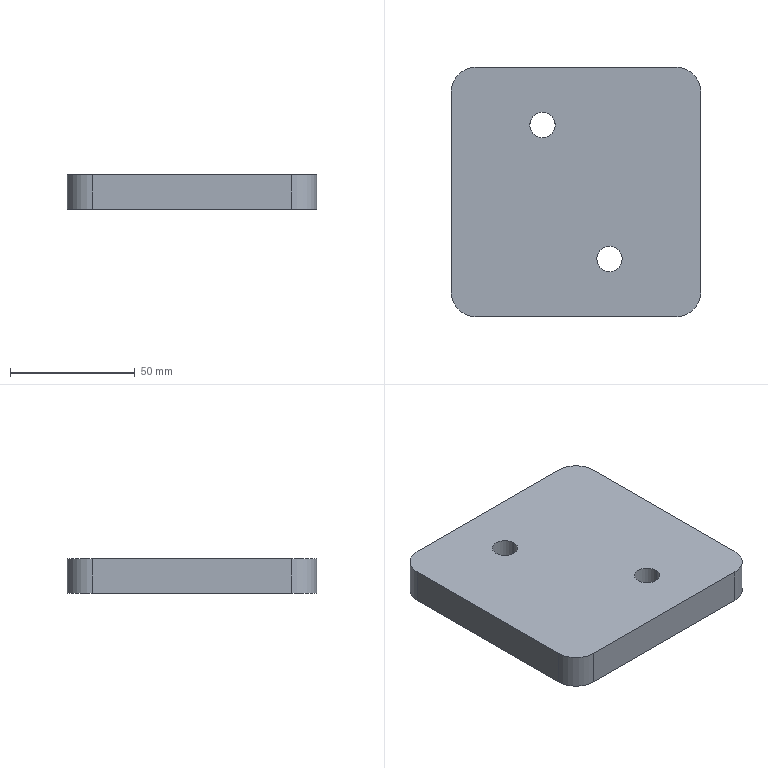Part | SolidWorks | features 3DProfileFeature 1, Extrusion 1, Fillet 1, HoleWzd 1 | 1 solid | 14 faces | box 100 x 100 x 14 mm | volume 136510 mm3 | cylinder 8 | plane 6 | commonest cylinder face diameters 10.2 x4 20 x4
STEP:
#1=CARTESIAN_POINT('',(-18.516,26.833,0.));
#2=VERTEX_POINT('',#1);
#3=CARTESIAN_POINT('',(-8.316,26.833,0.));
#4=VERTEX_POINT('',#3);
#5=CARTESIAN_POINT('',(-13.416,26.833,0.));
#6=DIRECTION('',(0.,0.,1.));
#7=DIRECTION('',(1.,0.,0.));
#8=AXIS2_PLACEMENT_3D('',#5,#6,#7);
#9=CIRCLE('',#8,5.1);
#10=EDGE_CURVE('',#2,#4,#9,.T.);
#11=ORIENTED_EDGE('',*,*,#10,.F.);
#12=CARTESIAN_POINT('',(-18.516,26.833,14.));
#13=VERTEX_POINT('',#12);
#14=CARTESIAN_POINT('',(-18.516,26.833,14.));
#15=DIRECTION('',(0.,0.,1.));
#16=VECTOR('',#15,1000.);
#17=LINE('',#14,#16);
#18=EDGE_CURVE('',#2,#13,#17,.T.);
#19=ORIENTED_EDGE('',*,*,#18,.T.);
#20=CARTESIAN_POINT('',(-8.316,26.833,14.));
#21=VERTEX_POINT('',#20);
#22=CARTESIAN_POINT('',(-13.416,26.833,14.));
#23=DIRECTION('',(0.,0.,1.));
#24=DIRECTION('',(1.,0.,0.));
#25=AXIS2_PLACEMENT_3D('',#22,#23,#24);
#26=CIRCLE('',#25,5.1);
#27=EDGE_CURVE('',#13,#21,#26,.T.);
#28=ORIENTED_EDGE('',*,*,#27,.T.);
#29=CARTESIAN_POINT('',(-8.316,26.833,14.));
#30=DIRECTION('',(0.,0.,1.));
#31=VECTOR('',#30,1000.);
#32=LINE('',#29,#31);
#33=EDGE_CURVE('',#4,#21,#32,.T.);
#34=ORIENTED_EDGE('',*,*,#33,.F.);
#35=EDGE_LOOP('',(#11,#19,#28,#34));
#36=FACE_OUTER_BOUND('',#35,.T.);
#37=CARTESIAN_POINT('',(-13.416,26.833,14.));
#38=DIRECTION('',(0.,0.,1.));
#39=DIRECTION('',(1.,0.,0.));
#40=AXIS2_PLACEMENT_3D('',#37,#38,#39);
#41=CYLINDRICAL_SURFACE('',#40,5.1);
#42=ADVANCED_FACE('',(#36),#41,.F.);
#43=CARTESIAN_POINT('',(8.316,-26.833,0.));
#44=VERTEX_POINT('',#43);
#45=CARTESIAN_POINT('',(18.516,-26.833,0.));
#46=VERTEX_POINT('',#45);
#47=CARTESIAN_POINT('',(13.416,-26.833,0.));
#48=DIRECTION('',(0.,0.,1.));
#49=DIRECTION('',(1.,0.,0.));
#50=AXIS2_PLACEMENT_3D('',#47,#48,#49);
#51=CIRCLE('',#50,5.1);
#52=EDGE_CURVE('',#44,#46,#51,.T.);
#53=ORIENTED_EDGE('',*,*,#52,.F.);
#54=CARTESIAN_POINT('',(8.316,-26.833,14.));
#55=VERTEX_POINT('',#54);
#56=CARTESIAN_POINT('',(8.316,-26.833,14.));
#57=DIRECTION('',(0.,0.,1.));
#58=VECTOR('',#57,1000.);
#59=LINE('',#56,#58);
#60=EDGE_CURVE('',#44,#55,#59,.T.);
#61=ORIENTED_EDGE('',*,*,#60,.T.);
#62=CARTESIAN_POINT('',(18.516,-26.833,14.));
#63=VERTEX_POINT('',#62);
#64=CARTESIAN_POINT('',(13.416,-26.833,14.));
#65=DIRECTION('',(0.,0.,1.));
#66=DIRECTION('',(1.,0.,0.));
#67=AXIS2_PLACEMENT_3D('',#64,#65,#66);
#68=CIRCLE('',#67,5.1);
#69=EDGE_CURVE('',#55,#63,#68,.T.);
#70=ORIENTED_EDGE('',*,*,#69,.T.);
#71=CARTESIAN_POINT('',(18.516,-26.833,14.));
#72=DIRECTION('',(0.,0.,1.));
#73=VECTOR('',#72,1000.);
#74=LINE('',#71,#73);
#75=EDGE_CURVE('',#46,#63,#74,.T.);
#76=ORIENTED_EDGE('',*,*,#75,.F.);
#77=EDGE_LOOP('',(#53,#61,#70,#76));
#78=FACE_OUTER_BOUND('',#77,.T.);
#79=CARTESIAN_POINT('',(13.416,-26.833,14.));
#80=DIRECTION('',(0.,0.,1.));
#81=DIRECTION('',(1.,0.,0.));
#82=AXIS2_PLACEMENT_3D('',#79,#80,#81);
#83=CYLINDRICAL_SURFACE('',#82,5.1);
#84=ADVANCED_FACE('',(#78),#83,.F.);
#85=CARTESIAN_POINT('',(-40.,50.,14.));
#86=VERTEX_POINT('',#85);
#87=CARTESIAN_POINT('',(40.,50.,14.));
#88=VERTEX_POINT('',#87);
#89=CARTESIAN_POINT('',(-50.,50.,14.));
#90=DIRECTION('',(1.,0.,0.));
#91=VECTOR('',#90,1000.);
#92=LINE('',#89,#91);
#93=EDGE_CURVE('',#86,#88,#92,.T.);
#94=ORIENTED_EDGE('',*,*,#93,.T.);
#95=CARTESIAN_POINT('',(40.,50.,0.));
#96=VERTEX_POINT('',#95);
#97=CARTESIAN_POINT('',(40.,50.,14.));
#98=DIRECTION('',(0.,0.,-1.));
#99=VECTOR('',#98,1000.);
#100=LINE('',#97,#99);
#101=EDGE_CURVE('',#88,#96,#100,.T.);
#102=ORIENTED_EDGE('',*,*,#101,.T.);
#103=CARTESIAN_POINT('',(-40.,50.,0.));
#104=VERTEX_POINT('',#103);
#105=CARTESIAN_POINT('',(-50.,50.,0.));
#106=DIRECTION('',(1.,0.,0.));
#107=VECTOR('',#106,1000.);
#108=LINE('',#105,#107);
#109=EDGE_CURVE('',#104,#96,#108,.T.);
#110=ORIENTED_EDGE('',*,*,#109,.F.);
#111=CARTESIAN_POINT('',(-40.,50.,14.));
#112=DIRECTION('',(0.,0.,1.));
#113=VECTOR('',#112,1000.);
#114=LINE('',#111,#113);
#115=EDGE_CURVE('',#104,#86,#114,.T.);
#116=ORIENTED_EDGE('',*,*,#115,.T.);
#117=EDGE_LOOP('',(#94,#102,#110,#116));
#118=FACE_OUTER_BOUND('',#117,.T.);
#119=CARTESIAN_POINT('',(-50.,50.,14.));
#120=DIRECTION('',(0.,1.,0.));
#121=DIRECTION('',(0.,0.,1.));
#122=AXIS2_PLACEMENT_3D('',#119,#120,#121);
#123=PLANE('',#122);
#124=ADVANCED_FACE('',(#118),#123,.T.);
#125=CARTESIAN_POINT('',(-50.,40.,0.));
#126=VERTEX_POINT('',#125);
#127=CARTESIAN_POINT('',(-50.,-40.,0.));
#128=VERTEX_POINT('',#127);
#129=CARTESIAN_POINT('',(-50.,50.,0.));
#130=DIRECTION('',(0.,-1.,0.));
#131=VECTOR('',#130,1000.);
#132=LINE('',#129,#131);
#133=EDGE_CURVE('',#126,#128,#132,.T.);
#134=ORIENTED_EDGE('',*,*,#133,.T.);
#135=CARTESIAN_POINT('',(-50.,-40.,14.));
#136=VERTEX_POINT('',#135);
#137=CARTESIAN_POINT('',(-50.,-40.,14.));
#138=DIRECTION('',(0.,0.,1.));
#139=VECTOR('',#138,1000.);
#140=LINE('',#137,#139);
#141=EDGE_CURVE('',#128,#136,#140,.T.);
#142=ORIENTED_EDGE('',*,*,#141,.T.);
#143=CARTESIAN_POINT('',(-50.,40.,14.));
#144=VERTEX_POINT('',#143);
#145=CARTESIAN_POINT('',(-50.,50.,14.));
#146=DIRECTION('',(0.,-1.,0.));
#147=VECTOR('',#146,1000.);
#148=LINE('',#145,#147);
#149=EDGE_CURVE('',#144,#136,#148,.T.);
#150=ORIENTED_EDGE('',*,*,#149,.F.);
#151=CARTESIAN_POINT('',(-50.,40.,0.));
#152=DIRECTION('',(0.,0.,-1.));
#153=VECTOR('',#152,1000.);
#154=LINE('',#151,#153);
#155=EDGE_CURVE('',#144,#126,#154,.T.);
#156=ORIENTED_EDGE('',*,*,#155,.T.);
#157=EDGE_LOOP('',(#134,#142,#150,#156));
#158=FACE_OUTER_BOUND('',#157,.T.);
#159=CARTESIAN_POINT('',(-50.,50.,14.));
#160=DIRECTION('',(1.,0.,0.));
#161=DIRECTION('',(0.,1.,0.));
#162=AXIS2_PLACEMENT_3D('',#159,#160,#161);
#163=PLANE('',#162);
#164=ADVANCED_FACE('',(#158),#163,.F.);
#165=CARTESIAN_POINT('',(-40.,-50.,0.));
#166=VERTEX_POINT('',#165);
#167=CARTESIAN_POINT('',(40.,-50.,0.));
#168=VERTEX_POINT('',#167);
#169=CARTESIAN_POINT('',(-50.,-50.,0.));
#170=DIRECTION('',(1.,0.,0.));
#171=VECTOR('',#170,1000.);
#172=LINE('',#169,#171);
#173=EDGE_CURVE('',#166,#168,#172,.T.);
#174=ORIENTED_EDGE('',*,*,#173,.T.);
#175=CARTESIAN_POINT('',(40.,-50.,14.));
#176=VERTEX_POINT('',#175);
#177=CARTESIAN_POINT('',(40.,-50.,14.));
#178=DIRECTION('',(0.,0.,1.));
#179=VECTOR('',#178,1000.);
#180=LINE('',#177,#179);
#181=EDGE_CURVE('',#168,#176,#180,.T.);
#182=ORIENTED_EDGE('',*,*,#181,.T.);
#183=CARTESIAN_POINT('',(-40.,-50.,14.));
#184=VERTEX_POINT('',#183);
#185=CARTESIAN_POINT('',(-50.,-50.,14.));
#186=DIRECTION('',(1.,0.,0.));
#187=VECTOR('',#186,1000.);
#188=LINE('',#185,#187);
#189=EDGE_CURVE('',#184,#176,#188,.T.);
#190=ORIENTED_EDGE('',*,*,#189,.F.);
#191=CARTESIAN_POINT('',(-40.,-50.,14.));
#192=DIRECTION('',(0.,0.,-1.));
#193=VECTOR('',#192,1000.);
#194=LINE('',#191,#193);
#195=EDGE_CURVE('',#184,#166,#194,.T.);
#196=ORIENTED_EDGE('',*,*,#195,.T.);
#197=EDGE_LOOP('',(#174,#182,#190,#196));
#198=FACE_OUTER_BOUND('',#197,.T.);
#199=CARTESIAN_POINT('',(-50.,-50.,14.));
#200=DIRECTION('',(0.,1.,0.));
#201=DIRECTION('',(0.,0.,1.));
#202=AXIS2_PLACEMENT_3D('',#199,#200,#201);
#203=PLANE('',#202);
#204=ADVANCED_FACE('',(#198),#203,.F.);
#205=CARTESIAN_POINT('',(50.,40.,14.));
#206=VERTEX_POINT('',#205);
#207=CARTESIAN_POINT('',(50.,-40.,14.));
#208=VERTEX_POINT('',#207);
#209=CARTESIAN_POINT('',(50.,50.,14.));
#210=DIRECTION('',(0.,-1.,0.));
#211=VECTOR('',#210,1000.);
#212=LINE('',#209,#211);
#213=EDGE_CURVE('',#206,#208,#212,.T.);
#214=ORIENTED_EDGE('',*,*,#213,.T.);
#215=CARTESIAN_POINT('',(50.,-40.,0.));
#216=VERTEX_POINT('',#215);
#217=CARTESIAN_POINT('',(50.,-40.,0.));
#218=DIRECTION('',(0.,0.,-1.));
#219=VECTOR('',#218,1000.);
#220=LINE('',#217,#219);
#221=EDGE_CURVE('',#208,#216,#220,.T.);
#222=ORIENTED_EDGE('',*,*,#221,.T.);
#223=CARTESIAN_POINT('',(50.,40.,0.));
#224=VERTEX_POINT('',#223);
#225=CARTESIAN_POINT('',(50.,50.,0.));
#226=DIRECTION('',(0.,-1.,0.));
#227=VECTOR('',#226,1000.);
#228=LINE('',#225,#227);
#229=EDGE_CURVE('',#224,#216,#228,.T.);
#230=ORIENTED_EDGE('',*,*,#229,.F.);
#231=CARTESIAN_POINT('',(50.,40.,14.));
#232=DIRECTION('',(0.,0.,1.));
#233=VECTOR('',#232,1000.);
#234=LINE('',#231,#233);
#235=EDGE_CURVE('',#224,#206,#234,.T.);
#236=ORIENTED_EDGE('',*,*,#235,.T.);
#237=EDGE_LOOP('',(#214,#222,#230,#236));
#238=FACE_OUTER_BOUND('',#237,.T.);
#239=CARTESIAN_POINT('',(50.,50.,14.));
#240=DIRECTION('',(1.,0.,0.));
#241=DIRECTION('',(0.,0.,-1.));
#242=AXIS2_PLACEMENT_3D('',#239,#240,#241);
#243=PLANE('',#242);
#244=ADVANCED_FACE('',(#238),#243,.T.);
#245=CARTESIAN_POINT('',(-13.416,26.833,14.));
#246=DIRECTION('',(0.,0.,1.));
#247=DIRECTION('',(1.,0.,0.));
#248=AXIS2_PLACEMENT_3D('',#245,#246,#247);
#249=CIRCLE('',#248,5.1);
#250=EDGE_CURVE('',#21,#13,#249,.T.);
#251=ORIENTED_EDGE('',*,*,#250,.F.);
#252=ORIENTED_EDGE('',*,*,#27,.F.);
#253=EDGE_LOOP('',(#251,#252));
#254=FACE_BOUND('',#253,.T.);
#255=CARTESIAN_POINT('',(13.416,-26.833,14.));
#256=DIRECTION('',(0.,0.,1.));
#257=DIRECTION('',(1.,0.,0.));
#258=AXIS2_PLACEMENT_3D('',#255,#256,#257);
#259=CIRCLE('',#258,5.1);
#260=EDGE_CURVE('',#63,#55,#259,.T.);
#261=ORIENTED_EDGE('',*,*,#260,.F.);
#262=ORIENTED_EDGE('',*,*,#69,.F.);
#263=EDGE_LOOP('',(#261,#262));
#264=FACE_BOUND('',#263,.T.);
#265=ORIENTED_EDGE('',*,*,#189,.T.);
#266=CARTESIAN_POINT('',(40.,-40.,14.));
#267=DIRECTION('',(0.,0.,1.));
#268=DIRECTION('',(-1.,0.,0.));
#269=AXIS2_PLACEMENT_3D('',#266,#267,#268);
#270=CIRCLE('',#269,10.);
#271=EDGE_CURVE('',#176,#208,#270,.T.);
#272=ORIENTED_EDGE('',*,*,#271,.T.);
#273=ORIENTED_EDGE('',*,*,#213,.F.);
#274=CARTESIAN_POINT('',(40.,40.,14.));
#275=DIRECTION('',(0.,0.,1.));
#276=DIRECTION('',(-1.,0.,0.));
#277=AXIS2_PLACEMENT_3D('',#274,#275,#276);
#278=CIRCLE('',#277,10.);
#279=EDGE_CURVE('',#206,#88,#278,.T.);
#280=ORIENTED_EDGE('',*,*,#279,.T.);
#281=ORIENTED_EDGE('',*,*,#93,.F.);
#282=CARTESIAN_POINT('',(-40.,40.,14.));
#283=DIRECTION('',(0.,0.,1.));
#284=DIRECTION('',(-1.,0.,0.));
#285=AXIS2_PLACEMENT_3D('',#282,#283,#284);
#286=CIRCLE('',#285,10.);
#287=EDGE_CURVE('',#86,#144,#286,.T.);
#288=ORIENTED_EDGE('',*,*,#287,.T.);
#289=ORIENTED_EDGE('',*,*,#149,.T.);
#290=CARTESIAN_POINT('',(-40.,-40.,14.));
#291=DIRECTION('',(0.,0.,1.));
#292=DIRECTION('',(-1.,0.,0.));
#293=AXIS2_PLACEMENT_3D('',#290,#291,#292);
#294=CIRCLE('',#293,10.);
#295=EDGE_CURVE('',#136,#184,#294,.T.);
#296=ORIENTED_EDGE('',*,*,#295,.T.);
#297=EDGE_LOOP('',(#265,#272,#273,#280,#281,#288,#289,#296));
#298=FACE_OUTER_BOUND('',#297,.T.);
#299=CARTESIAN_POINT('',(0.,0.,14.));
#300=DIRECTION('',(0.,0.,-1.));
#301=DIRECTION('',(-1.,0.,0.));
#302=AXIS2_PLACEMENT_3D('',#299,#300,#301);
#303=PLANE('',#302);
#304=ADVANCED_FACE('',(#254,#264,#298),#303,.F.);
#305=CARTESIAN_POINT('',(-13.416,26.833,0.));
#306=DIRECTION('',(0.,0.,1.));
#307=DIRECTION('',(1.,0.,0.));
#308=AXIS2_PLACEMENT_3D('',#305,#306,#307);
#309=CIRCLE('',#308,5.1);
#310=EDGE_CURVE('',#4,#2,#309,.T.);
#311=ORIENTED_EDGE('',*,*,#310,.T.);
#312=ORIENTED_EDGE('',*,*,#10,.T.);
#313=EDGE_LOOP('',(#311,#312));
#314=FACE_BOUND('',#313,.T.);
#315=CARTESIAN_POINT('',(13.416,-26.833,0.));
#316=DIRECTION('',(0.,0.,1.));
#317=DIRECTION('',(1.,0.,0.));
#318=AXIS2_PLACEMENT_3D('',#315,#316,#317);
#319=CIRCLE('',#318,5.1);
#320=EDGE_CURVE('',#46,#44,#319,.T.);
#321=ORIENTED_EDGE('',*,*,#320,.T.);
#322=ORIENTED_EDGE('',*,*,#52,.T.);
#323=EDGE_LOOP('',(#321,#322));
#324=FACE_BOUND('',#323,.T.);
#325=ORIENTED_EDGE('',*,*,#229,.T.);
#326=CARTESIAN_POINT('',(40.,-40.,0.));
#327=DIRECTION('',(0.,0.,-1.));
#328=DIRECTION('',(-1.,0.,0.));
#329=AXIS2_PLACEMENT_3D('',#326,#327,#328);
#330=CIRCLE('',#329,10.);
#331=EDGE_CURVE('',#216,#168,#330,.T.);
#332=ORIENTED_EDGE('',*,*,#331,.T.);
#333=ORIENTED_EDGE('',*,*,#173,.F.);
#334=CARTESIAN_POINT('',(-40.,-40.,0.));
#335=DIRECTION('',(0.,0.,-1.));
#336=DIRECTION('',(-1.,0.,0.));
#337=AXIS2_PLACEMENT_3D('',#334,#335,#336);
#338=CIRCLE('',#337,10.);
#339=EDGE_CURVE('',#166,#128,#338,.T.);
#340=ORIENTED_EDGE('',*,*,#339,.T.);
#341=ORIENTED_EDGE('',*,*,#133,.F.);
#342=CARTESIAN_POINT('',(-40.,40.,0.));
#343=DIRECTION('',(0.,0.,-1.));
#344=DIRECTION('',(-1.,0.,0.));
#345=AXIS2_PLACEMENT_3D('',#342,#343,#344);
#346=CIRCLE('',#345,10.);
#347=EDGE_CURVE('',#126,#104,#346,.T.);
#348=ORIENTED_EDGE('',*,*,#347,.T.);
#349=ORIENTED_EDGE('',*,*,#109,.T.);
#350=CARTESIAN_POINT('',(40.,40.,0.));
#351=DIRECTION('',(0.,0.,-1.));
#352=DIRECTION('',(-1.,0.,0.));
#353=AXIS2_PLACEMENT_3D('',#350,#351,#352);
#354=CIRCLE('',#353,10.);
#355=EDGE_CURVE('',#96,#224,#354,.T.);
#356=ORIENTED_EDGE('',*,*,#355,.T.);
#357=EDGE_LOOP('',(#325,#332,#333,#340,#341,#348,#349,#356));
#358=FACE_OUTER_BOUND('',#357,.T.);
#359=CARTESIAN_POINT('',(0.,0.,0.));
#360=DIRECTION('',(0.,0.,-1.));
#361=DIRECTION('',(-1.,0.,0.));
#362=AXIS2_PLACEMENT_3D('',#359,#360,#361);
#363=PLANE('',#362);
#364=ADVANCED_FACE('',(#314,#324,#358),#363,.T.);
#365=ORIENTED_EDGE('',*,*,#60,.F.);
#366=ORIENTED_EDGE('',*,*,#320,.F.);
#367=ORIENTED_EDGE('',*,*,#75,.T.);
#368=ORIENTED_EDGE('',*,*,#260,.T.);
#369=EDGE_LOOP('',(#365,#366,#367,#368));
#370=FACE_OUTER_BOUND('',#369,.T.);
#371=CARTESIAN_POINT('',(13.416,-26.833,14.));
#372=DIRECTION('',(0.,0.,1.));
#373=DIRECTION('',(1.,0.,0.));
#374=AXIS2_PLACEMENT_3D('',#371,#372,#373);
#375=CYLINDRICAL_SURFACE('',#374,5.1);
#376=ADVANCED_FACE('',(#370),#375,.F.);
#377=ORIENTED_EDGE('',*,*,#18,.F.);
#378=ORIENTED_EDGE('',*,*,#310,.F.);
#379=ORIENTED_EDGE('',*,*,#33,.T.);
#380=ORIENTED_EDGE('',*,*,#250,.T.);
#381=EDGE_LOOP('',(#377,#378,#379,#380));
#382=FACE_OUTER_BOUND('',#381,.T.);
#383=CARTESIAN_POINT('',(-13.416,26.833,14.));
#384=DIRECTION('',(0.,0.,1.));
#385=DIRECTION('',(1.,0.,0.));
#386=AXIS2_PLACEMENT_3D('',#383,#384,#385);
#387=CYLINDRICAL_SURFACE('',#386,5.1);
#388=ADVANCED_FACE('',(#382),#387,.F.);
#389=ORIENTED_EDGE('',*,*,#271,.F.);
#390=ORIENTED_EDGE('',*,*,#181,.F.);
#391=ORIENTED_EDGE('',*,*,#331,.F.);
#392=ORIENTED_EDGE('',*,*,#221,.F.);
#393=EDGE_LOOP('',(#389,#390,#391,#392));
#394=FACE_OUTER_BOUND('',#393,.T.);
#395=CARTESIAN_POINT('',(40.,-40.,14.));
#396=DIRECTION('',(0.,0.,1.));
#397=DIRECTION('',(1.,0.,0.));
#398=AXIS2_PLACEMENT_3D('',#395,#396,#397);
#399=CYLINDRICAL_SURFACE('',#398,10.);
#400=ADVANCED_FACE('',(#394),#399,.T.);
#401=ORIENTED_EDGE('',*,*,#295,.F.);
#402=ORIENTED_EDGE('',*,*,#141,.F.);
#403=ORIENTED_EDGE('',*,*,#339,.F.);
#404=ORIENTED_EDGE('',*,*,#195,.F.);
#405=EDGE_LOOP('',(#401,#402,#403,#404));
#406=FACE_OUTER_BOUND('',#405,.T.);
#407=CARTESIAN_POINT('',(-40.,-40.,14.));
#408=DIRECTION('',(0.,0.,-1.));
#409=DIRECTION('',(-1.,0.,0.));
#410=AXIS2_PLACEMENT_3D('',#407,#408,#409);
#411=CYLINDRICAL_SURFACE('',#410,10.);
#412=ADVANCED_FACE('',(#406),#411,.T.);
#413=ORIENTED_EDGE('',*,*,#279,.F.);
#414=ORIENTED_EDGE('',*,*,#235,.F.);
#415=ORIENTED_EDGE('',*,*,#355,.F.);
#416=ORIENTED_EDGE('',*,*,#101,.F.);
#417=EDGE_LOOP('',(#413,#414,#415,#416));
#418=FACE_OUTER_BOUND('',#417,.T.);
#419=CARTESIAN_POINT('',(40.,40.,14.));
#420=DIRECTION('',(0.,0.,-1.));
#421=DIRECTION('',(-1.,0.,0.));
#422=AXIS2_PLACEMENT_3D('',#419,#420,#421);
#423=CYLINDRICAL_SURFACE('',#422,10.);
#424=ADVANCED_FACE('',(#418),#423,.T.);
#425=ORIENTED_EDGE('',*,*,#287,.F.);
#426=ORIENTED_EDGE('',*,*,#115,.F.);
#427=ORIENTED_EDGE('',*,*,#347,.F.);
#428=ORIENTED_EDGE('',*,*,#155,.F.);
#429=EDGE_LOOP('',(#425,#426,#427,#428));
#430=FACE_OUTER_BOUND('',#429,.T.);
#431=CARTESIAN_POINT('',(-40.,40.,14.));
#432=DIRECTION('',(0.,0.,1.));
#433=DIRECTION('',(1.,0.,0.));
#434=AXIS2_PLACEMENT_3D('',#431,#432,#433);
#435=CYLINDRICAL_SURFACE('',#434,10.);
#436=ADVANCED_FACE('',(#430),#435,.T.);
#437=CLOSED_SHELL('',(#42,#84,#124,#164,#204,#244,#304,#364,#376,#388,#400,#412,#424,#436));
#438=MANIFOLD_SOLID_BREP('',#437);
#439=CARTESIAN_POINT('',(0.,0.,0.));
#440=DIRECTION('',(0.,0.,1.));
#441=DIRECTION('',(1.,0.,0.));
#442=AXIS2_PLACEMENT_3D('',#439,#440,#441);
#443=(LENGTH_UNIT()NAMED_UNIT(*)SI_UNIT(.MILLI.,.METRE.));
#444=UNCERTAINTY_MEASURE_WITH_UNIT(LENGTH_MEASURE(0.00001),#443,'','');
#445=(NAMED_UNIT(*)PLANE_ANGLE_UNIT()SI_UNIT($,.RADIAN.));
#446=(NAMED_UNIT(*)SI_UNIT($,.STERADIAN.)SOLID_ANGLE_UNIT());
#447=(GEOMETRIC_REPRESENTATION_CONTEXT(3)GLOBAL_UNCERTAINTY_ASSIGNED_CONTEXT((#444))GLOBAL_UNIT_ASSIGNED_CONTEXT((#443,#445,#446))REPRESENTATION_CONTEXT('',''));
#448=ADVANCED_BREP_SHAPE_REPRESENTATION('',(#438,#442),#447);